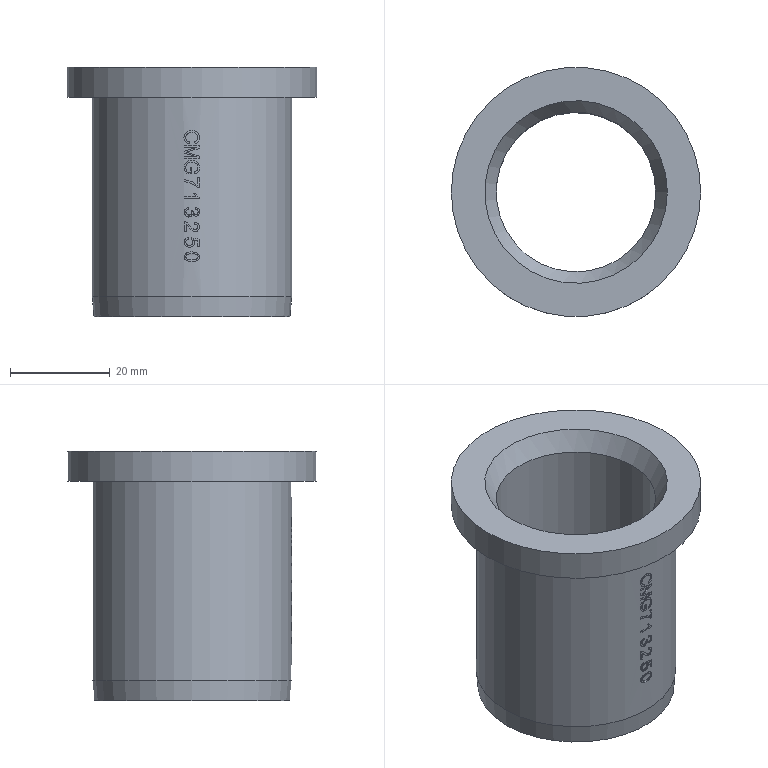Part | NX | features 18 2 | 1 solid | 84 faces | box 50 x 50 x 50 mm | volume 26196 mm3 | plane 48 | spline 20 | cylinder 13 | cone 2 | torus 1 | commonest cylinder face diameters 39.8 x9 40 x2 32 x1 50 x1